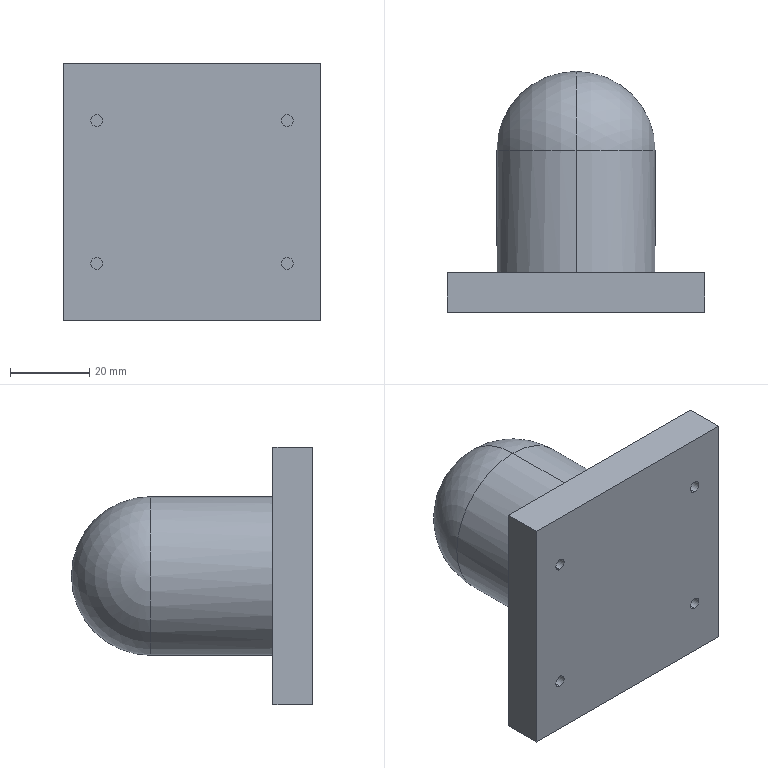Part | SolidWorks | features ICE 2, Extrusion 1, Fillet 1 | 1 solid | 22 faces | box 65 x 60.8 x 65 mm | volume 97568 mm3 | cylinder 10 | plane 10 | sphere 2 | commonest cylinder face diameters 3 x8 40 x2
STEP:
#1=CARTESIAN_POINT('',(24.,5.,-16.5));
#2=VERTEX_POINT('',#1);
#3=CARTESIAN_POINT('',(24.,5.,-19.5));
#4=VERTEX_POINT('',#3);
#5=CARTESIAN_POINT('',(24.,5.,-18.));
#6=DIRECTION('',(0.,-1.,0.));
#7=DIRECTION('',(0.,0.,-1.));
#8=AXIS2_PLACEMENT_3D('',#5,#6,#7);
#9=CIRCLE('',#8,1.5);
#10=EDGE_CURVE('',#2,#4,#9,.T.);
#11=ORIENTED_EDGE('',*,*,#10,.F.);
#12=CARTESIAN_POINT('',(24.,0.,-16.5));
#13=VERTEX_POINT('',#12);
#14=CARTESIAN_POINT('',(24.,5.,-16.5));
#15=DIRECTION('',(0.,-1.,0.));
#16=VECTOR('',#15,1000.);
#17=LINE('',#14,#16);
#18=EDGE_CURVE('',#2,#13,#17,.T.);
#19=ORIENTED_EDGE('',*,*,#18,.T.);
#20=CARTESIAN_POINT('',(24.,0.,-19.5));
#21=VERTEX_POINT('',#20);
#22=CARTESIAN_POINT('',(24.,0.,-18.));
#23=DIRECTION('',(0.,-1.,0.));
#24=DIRECTION('',(0.,0.,-1.));
#25=AXIS2_PLACEMENT_3D('',#22,#23,#24);
#26=CIRCLE('',#25,1.5);
#27=EDGE_CURVE('',#13,#21,#26,.T.);
#28=ORIENTED_EDGE('',*,*,#27,.T.);
#29=CARTESIAN_POINT('',(24.,5.,-19.5));
#30=DIRECTION('',(0.,-1.,0.));
#31=VECTOR('',#30,1000.);
#32=LINE('',#29,#31);
#33=EDGE_CURVE('',#4,#21,#32,.T.);
#34=ORIENTED_EDGE('',*,*,#33,.F.);
#35=EDGE_LOOP('',(#11,#19,#28,#34));
#36=FACE_OUTER_BOUND('',#35,.T.);
#37=CARTESIAN_POINT('',(24.,5.,-18.));
#38=DIRECTION('',(0.,-1.,0.));
#39=DIRECTION('',(0.,0.,-1.));
#40=AXIS2_PLACEMENT_3D('',#37,#38,#39);
#41=CYLINDRICAL_SURFACE('',#40,1.5);
#42=ADVANCED_FACE('',(#36),#41,.F.);
#43=CARTESIAN_POINT('',(-24.,5.,-16.5));
#44=VERTEX_POINT('',#43);
#45=CARTESIAN_POINT('',(-24.,5.,-19.5));
#46=VERTEX_POINT('',#45);
#47=CARTESIAN_POINT('',(-24.,5.,-18.));
#48=DIRECTION('',(0.,-1.,0.));
#49=DIRECTION('',(0.,0.,-1.));
#50=AXIS2_PLACEMENT_3D('',#47,#48,#49);
#51=CIRCLE('',#50,1.5);
#52=EDGE_CURVE('',#44,#46,#51,.T.);
#53=ORIENTED_EDGE('',*,*,#52,.F.);
#54=CARTESIAN_POINT('',(-24.,0.,-16.5));
#55=VERTEX_POINT('',#54);
#56=CARTESIAN_POINT('',(-24.,5.,-16.5));
#57=DIRECTION('',(0.,-1.,0.));
#58=VECTOR('',#57,1000.);
#59=LINE('',#56,#58);
#60=EDGE_CURVE('',#44,#55,#59,.T.);
#61=ORIENTED_EDGE('',*,*,#60,.T.);
#62=CARTESIAN_POINT('',(-24.,0.,-19.5));
#63=VERTEX_POINT('',#62);
#64=CARTESIAN_POINT('',(-24.,0.,-18.));
#65=DIRECTION('',(0.,-1.,0.));
#66=DIRECTION('',(0.,0.,-1.));
#67=AXIS2_PLACEMENT_3D('',#64,#65,#66);
#68=CIRCLE('',#67,1.5);
#69=EDGE_CURVE('',#55,#63,#68,.T.);
#70=ORIENTED_EDGE('',*,*,#69,.T.);
#71=CARTESIAN_POINT('',(-24.,5.,-19.5));
#72=DIRECTION('',(0.,-1.,0.));
#73=VECTOR('',#72,1000.);
#74=LINE('',#71,#73);
#75=EDGE_CURVE('',#46,#63,#74,.T.);
#76=ORIENTED_EDGE('',*,*,#75,.F.);
#77=EDGE_LOOP('',(#53,#61,#70,#76));
#78=FACE_OUTER_BOUND('',#77,.T.);
#79=CARTESIAN_POINT('',(-24.,5.,-18.));
#80=DIRECTION('',(0.,-1.,0.));
#81=DIRECTION('',(0.,0.,-1.));
#82=AXIS2_PLACEMENT_3D('',#79,#80,#81);
#83=CYLINDRICAL_SURFACE('',#82,1.5);
#84=ADVANCED_FACE('',(#78),#83,.F.);
#85=CARTESIAN_POINT('',(-24.,5.,19.5));
#86=VERTEX_POINT('',#85);
#87=CARTESIAN_POINT('',(-24.,5.,16.5));
#88=VERTEX_POINT('',#87);
#89=CARTESIAN_POINT('',(-24.,5.,18.));
#90=DIRECTION('',(0.,-1.,0.));
#91=DIRECTION('',(0.,0.,-1.));
#92=AXIS2_PLACEMENT_3D('',#89,#90,#91);
#93=CIRCLE('',#92,1.5);
#94=EDGE_CURVE('',#86,#88,#93,.T.);
#95=ORIENTED_EDGE('',*,*,#94,.F.);
#96=CARTESIAN_POINT('',(-24.,0.,19.5));
#97=VERTEX_POINT('',#96);
#98=CARTESIAN_POINT('',(-24.,5.,19.5));
#99=DIRECTION('',(0.,-1.,0.));
#100=VECTOR('',#99,1000.);
#101=LINE('',#98,#100);
#102=EDGE_CURVE('',#86,#97,#101,.T.);
#103=ORIENTED_EDGE('',*,*,#102,.T.);
#104=CARTESIAN_POINT('',(-24.,0.,16.5));
#105=VERTEX_POINT('',#104);
#106=CARTESIAN_POINT('',(-24.,0.,18.));
#107=DIRECTION('',(0.,-1.,0.));
#108=DIRECTION('',(0.,0.,-1.));
#109=AXIS2_PLACEMENT_3D('',#106,#107,#108);
#110=CIRCLE('',#109,1.5);
#111=EDGE_CURVE('',#97,#105,#110,.T.);
#112=ORIENTED_EDGE('',*,*,#111,.T.);
#113=CARTESIAN_POINT('',(-24.,5.,16.5));
#114=DIRECTION('',(0.,-1.,0.));
#115=VECTOR('',#114,1000.);
#116=LINE('',#113,#115);
#117=EDGE_CURVE('',#88,#105,#116,.T.);
#118=ORIENTED_EDGE('',*,*,#117,.F.);
#119=EDGE_LOOP('',(#95,#103,#112,#118));
#120=FACE_OUTER_BOUND('',#119,.T.);
#121=CARTESIAN_POINT('',(-24.,5.,18.));
#122=DIRECTION('',(0.,-1.,0.));
#123=DIRECTION('',(0.,0.,-1.));
#124=AXIS2_PLACEMENT_3D('',#121,#122,#123);
#125=CYLINDRICAL_SURFACE('',#124,1.5);
#126=ADVANCED_FACE('',(#120),#125,.F.);
#127=CARTESIAN_POINT('',(24.,5.,19.5));
#128=VERTEX_POINT('',#127);
#129=CARTESIAN_POINT('',(24.,5.,16.5));
#130=VERTEX_POINT('',#129);
#131=CARTESIAN_POINT('',(24.,5.,18.));
#132=DIRECTION('',(0.,-1.,0.));
#133=DIRECTION('',(0.,0.,-1.));
#134=AXIS2_PLACEMENT_3D('',#131,#132,#133);
#135=CIRCLE('',#134,1.5);
#136=EDGE_CURVE('',#128,#130,#135,.T.);
#137=ORIENTED_EDGE('',*,*,#136,.F.);
#138=CARTESIAN_POINT('',(24.,0.,19.5));
#139=VERTEX_POINT('',#138);
#140=CARTESIAN_POINT('',(24.,5.,19.5));
#141=DIRECTION('',(0.,-1.,0.));
#142=VECTOR('',#141,1000.);
#143=LINE('',#140,#142);
#144=EDGE_CURVE('',#128,#139,#143,.T.);
#145=ORIENTED_EDGE('',*,*,#144,.T.);
#146=CARTESIAN_POINT('',(24.,0.,16.5));
#147=VERTEX_POINT('',#146);
#148=CARTESIAN_POINT('',(24.,0.,18.));
#149=DIRECTION('',(0.,-1.,0.));
#150=DIRECTION('',(0.,0.,-1.));
#151=AXIS2_PLACEMENT_3D('',#148,#149,#150);
#152=CIRCLE('',#151,1.5);
#153=EDGE_CURVE('',#139,#147,#152,.T.);
#154=ORIENTED_EDGE('',*,*,#153,.T.);
#155=CARTESIAN_POINT('',(24.,5.,16.5));
#156=DIRECTION('',(0.,-1.,0.));
#157=VECTOR('',#156,1000.);
#158=LINE('',#155,#157);
#159=EDGE_CURVE('',#130,#147,#158,.T.);
#160=ORIENTED_EDGE('',*,*,#159,.F.);
#161=EDGE_LOOP('',(#137,#145,#154,#160));
#162=FACE_OUTER_BOUND('',#161,.T.);
#163=CARTESIAN_POINT('',(24.,5.,18.));
#164=DIRECTION('',(0.,-1.,0.));
#165=DIRECTION('',(0.,0.,-1.));
#166=AXIS2_PLACEMENT_3D('',#163,#164,#165);
#167=CYLINDRICAL_SURFACE('',#166,1.5);
#168=ADVANCED_FACE('',(#162),#167,.F.);
#169=CARTESIAN_POINT('',(0.,40.8,-20.));
#170=VERTEX_POINT('',#169);
#171=CARTESIAN_POINT('',(0.,40.8,20.));
#172=VERTEX_POINT('',#171);
#173=CARTESIAN_POINT('',(0.,40.8,0.));
#174=DIRECTION('',(0.,-1.,0.));
#175=DIRECTION('',(0.,0.,-1.));
#176=AXIS2_PLACEMENT_3D('',#173,#174,#175);
#177=CIRCLE('',#176,20.);
#178=EDGE_CURVE('',#170,#172,#177,.T.);
#179=ORIENTED_EDGE('',*,*,#178,.F.);
#180=CARTESIAN_POINT('',(0.,60.8,0.));
#181=VERTEX_POINT('',#180);
#182=CARTESIAN_POINT('',(0.,40.8,0.));
#183=DIRECTION('',(1.,0.,0.));
#184=DIRECTION('',(0.,0.,-1.));
#185=AXIS2_PLACEMENT_3D('',#182,#183,#184);
#186=CIRCLE('',#185,20.);
#187=EDGE_CURVE('',#170,#181,#186,.T.);
#188=ORIENTED_EDGE('',*,*,#187,.T.);
#189=CARTESIAN_POINT('',(0.,40.8,0.));
#190=DIRECTION('',(-1.,0.,0.));
#191=DIRECTION('',(0.,0.,1.));
#192=AXIS2_PLACEMENT_3D('',#189,#190,#191);
#193=CIRCLE('',#192,20.);
#194=EDGE_CURVE('',#172,#181,#193,.T.);
#195=ORIENTED_EDGE('',*,*,#194,.F.);
#196=EDGE_LOOP('',(#179,#188,#195));
#197=FACE_OUTER_BOUND('',#196,.T.);
#198=CARTESIAN_POINT('',(0.,40.8,0.));
#199=DIRECTION('',(1.,0.,0.));
#200=DIRECTION('',(0.,0.,1.));
#201=AXIS2_PLACEMENT_3D('',#198,#199,#200);
#202=SPHERICAL_SURFACE('',#201,20.);
#203=ADVANCED_FACE('',(#197),#202,.T.);
#204=ORIENTED_EDGE('',*,*,#178,.T.);
#205=CARTESIAN_POINT('',(0.,10.,20.));
#206=VERTEX_POINT('',#205);
#207=CARTESIAN_POINT('',(0.,60.8,20.));
#208=DIRECTION('',(0.,-1.,0.));
#209=VECTOR('',#208,1000.);
#210=LINE('',#207,#209);
#211=EDGE_CURVE('',#172,#206,#210,.T.);
#212=ORIENTED_EDGE('',*,*,#211,.T.);
#213=CARTESIAN_POINT('',(0.,10.,-20.));
#214=VERTEX_POINT('',#213);
#215=CARTESIAN_POINT('',(0.,10.,0.));
#216=DIRECTION('',(0.,1.,0.));
#217=DIRECTION('',(0.,0.,1.));
#218=AXIS2_PLACEMENT_3D('',#215,#216,#217);
#219=CIRCLE('',#218,20.);
#220=EDGE_CURVE('',#206,#214,#219,.T.);
#221=ORIENTED_EDGE('',*,*,#220,.T.);
#222=CARTESIAN_POINT('',(0.,60.8,-20.));
#223=DIRECTION('',(0.,-1.,0.));
#224=VECTOR('',#223,1000.);
#225=LINE('',#222,#224);
#226=EDGE_CURVE('',#170,#214,#225,.T.);
#227=ORIENTED_EDGE('',*,*,#226,.F.);
#228=EDGE_LOOP('',(#204,#212,#221,#227));
#229=FACE_OUTER_BOUND('',#228,.T.);
#230=CARTESIAN_POINT('',(0.,60.8,0.));
#231=DIRECTION('',(0.,-1.,0.));
#232=DIRECTION('',(0.,0.,-1.));
#233=AXIS2_PLACEMENT_3D('',#230,#231,#232);
#234=CYLINDRICAL_SURFACE('',#233,20.);
#235=ADVANCED_FACE('',(#229),#234,.T.);
#236=CARTESIAN_POINT('',(32.5,0.,32.5));
#237=VERTEX_POINT('',#236);
#238=CARTESIAN_POINT('',(32.5,0.,-32.5));
#239=VERTEX_POINT('',#238);
#240=CARTESIAN_POINT('',(32.5,0.,32.5));
#241=DIRECTION('',(0.,0.,-1.));
#242=VECTOR('',#241,1000.);
#243=LINE('',#240,#242);
#244=EDGE_CURVE('',#237,#239,#243,.T.);
#245=ORIENTED_EDGE('',*,*,#244,.T.);
#246=CARTESIAN_POINT('',(32.5,10.,-32.5));
#247=VERTEX_POINT('',#246);
#248=CARTESIAN_POINT('',(32.5,10.,-32.5));
#249=DIRECTION('',(0.,-1.,0.));
#250=VECTOR('',#249,1000.);
#251=LINE('',#248,#250);
#252=EDGE_CURVE('',#247,#239,#251,.T.);
#253=ORIENTED_EDGE('',*,*,#252,.F.);
#254=CARTESIAN_POINT('',(32.5,10.,32.5));
#255=VERTEX_POINT('',#254);
#256=CARTESIAN_POINT('',(32.5,10.,32.5));
#257=DIRECTION('',(0.,0.,-1.));
#258=VECTOR('',#257,1000.);
#259=LINE('',#256,#258);
#260=EDGE_CURVE('',#255,#247,#259,.T.);
#261=ORIENTED_EDGE('',*,*,#260,.F.);
#262=CARTESIAN_POINT('',(32.5,10.,32.5));
#263=DIRECTION('',(0.,-1.,0.));
#264=VECTOR('',#263,1000.);
#265=LINE('',#262,#264);
#266=EDGE_CURVE('',#255,#237,#265,.T.);
#267=ORIENTED_EDGE('',*,*,#266,.T.);
#268=EDGE_LOOP('',(#245,#253,#261,#267));
#269=FACE_OUTER_BOUND('',#268,.T.);
#270=CARTESIAN_POINT('',(32.5,10.,32.5));
#271=DIRECTION('',(-1.,0.,0.));
#272=DIRECTION('',(0.,0.,1.));
#273=AXIS2_PLACEMENT_3D('',#270,#271,#272);
#274=PLANE('',#273);
#275=ADVANCED_FACE('',(#269),#274,.F.);
#276=CARTESIAN_POINT('',(-32.5,0.,-32.5));
#277=VERTEX_POINT('',#276);
#278=CARTESIAN_POINT('',(-32.5,0.,-32.5));
#279=DIRECTION('',(-1.,0.,0.));
#280=VECTOR('',#279,1000.);
#281=LINE('',#278,#280);
#282=EDGE_CURVE('',#239,#277,#281,.T.);
#283=ORIENTED_EDGE('',*,*,#282,.T.);
#284=CARTESIAN_POINT('',(-32.5,10.,-32.5));
#285=VERTEX_POINT('',#284);
#286=CARTESIAN_POINT('',(-32.5,10.,-32.5));
#287=DIRECTION('',(0.,-1.,0.));
#288=VECTOR('',#287,1000.);
#289=LINE('',#286,#288);
#290=EDGE_CURVE('',#285,#277,#289,.T.);
#291=ORIENTED_EDGE('',*,*,#290,.F.);
#292=CARTESIAN_POINT('',(-32.5,10.,-32.5));
#293=DIRECTION('',(-1.,0.,0.));
#294=VECTOR('',#293,1000.);
#295=LINE('',#292,#294);
#296=EDGE_CURVE('',#247,#285,#295,.T.);
#297=ORIENTED_EDGE('',*,*,#296,.F.);
#298=ORIENTED_EDGE('',*,*,#252,.T.);
#299=EDGE_LOOP('',(#283,#291,#297,#298));
#300=FACE_OUTER_BOUND('',#299,.T.);
#301=CARTESIAN_POINT('',(-32.5,10.,-32.5));
#302=DIRECTION('',(0.,0.,1.));
#303=DIRECTION('',(1.,0.,0.));
#304=AXIS2_PLACEMENT_3D('',#301,#302,#303);
#305=PLANE('',#304);
#306=ADVANCED_FACE('',(#300),#305,.F.);
#307=CARTESIAN_POINT('',(-32.5,0.,32.5));
#308=VERTEX_POINT('',#307);
#309=CARTESIAN_POINT('',(-32.5,0.,32.5));
#310=DIRECTION('',(0.,0.,1.));
#311=VECTOR('',#310,1000.);
#312=LINE('',#309,#311);
#313=EDGE_CURVE('',#277,#308,#312,.T.);
#314=ORIENTED_EDGE('',*,*,#313,.T.);
#315=CARTESIAN_POINT('',(-32.5,10.,32.5));
#316=VERTEX_POINT('',#315);
#317=CARTESIAN_POINT('',(-32.5,10.,32.5));
#318=DIRECTION('',(0.,-1.,0.));
#319=VECTOR('',#318,1000.);
#320=LINE('',#317,#319);
#321=EDGE_CURVE('',#316,#308,#320,.T.);
#322=ORIENTED_EDGE('',*,*,#321,.F.);
#323=CARTESIAN_POINT('',(-32.5,10.,32.5));
#324=DIRECTION('',(0.,0.,1.));
#325=VECTOR('',#324,1000.);
#326=LINE('',#323,#325);
#327=EDGE_CURVE('',#285,#316,#326,.T.);
#328=ORIENTED_EDGE('',*,*,#327,.F.);
#329=ORIENTED_EDGE('',*,*,#290,.T.);
#330=EDGE_LOOP('',(#314,#322,#328,#329));
#331=FACE_OUTER_BOUND('',#330,.T.);
#332=CARTESIAN_POINT('',(-32.5,10.,32.5));
#333=DIRECTION('',(1.,0.,0.));
#334=DIRECTION('',(0.,0.,-1.));
#335=AXIS2_PLACEMENT_3D('',#332,#333,#334);
#336=PLANE('',#335);
#337=ADVANCED_FACE('',(#331),#336,.F.);
#338=CARTESIAN_POINT('',(-32.5,0.,32.5));
#339=DIRECTION('',(1.,0.,0.));
#340=VECTOR('',#339,1000.);
#341=LINE('',#338,#340);
#342=EDGE_CURVE('',#308,#237,#341,.T.);
#343=ORIENTED_EDGE('',*,*,#342,.T.);
#344=ORIENTED_EDGE('',*,*,#266,.F.);
#345=CARTESIAN_POINT('',(-32.5,10.,32.5));
#346=DIRECTION('',(1.,0.,0.));
#347=VECTOR('',#346,1000.);
#348=LINE('',#345,#347);
#349=EDGE_CURVE('',#316,#255,#348,.T.);
#350=ORIENTED_EDGE('',*,*,#349,.F.);
#351=ORIENTED_EDGE('',*,*,#321,.T.);
#352=EDGE_LOOP('',(#343,#344,#350,#351));
#353=FACE_OUTER_BOUND('',#352,.T.);
#354=CARTESIAN_POINT('',(-32.5,10.,32.5));
#355=DIRECTION('',(0.,0.,-1.));
#356=DIRECTION('',(-1.,0.,0.));
#357=AXIS2_PLACEMENT_3D('',#354,#355,#356);
#358=PLANE('',#357);
#359=ADVANCED_FACE('',(#353),#358,.F.);
#360=CARTESIAN_POINT('',(0.,10.,0.));
#361=DIRECTION('',(0.,1.,0.));
#362=DIRECTION('',(0.,0.,1.));
#363=AXIS2_PLACEMENT_3D('',#360,#361,#362);
#364=CIRCLE('',#363,20.);
#365=EDGE_CURVE('',#214,#206,#364,.T.);
#366=ORIENTED_EDGE('',*,*,#365,.F.);
#367=ORIENTED_EDGE('',*,*,#220,.F.);
#368=EDGE_LOOP('',(#366,#367));
#369=FACE_BOUND('',#368,.T.);
#370=ORIENTED_EDGE('',*,*,#260,.T.);
#371=ORIENTED_EDGE('',*,*,#296,.T.);
#372=ORIENTED_EDGE('',*,*,#327,.T.);
#373=ORIENTED_EDGE('',*,*,#349,.T.);
#374=EDGE_LOOP('',(#370,#371,#372,#373));
#375=FACE_OUTER_BOUND('',#374,.T.);
#376=CARTESIAN_POINT('',(0.,10.,0.));
#377=DIRECTION('',(0.,-1.,0.));
#378=DIRECTION('',(0.,0.,-1.));
#379=AXIS2_PLACEMENT_3D('',#376,#377,#378);
#380=PLANE('',#379);
#381=ADVANCED_FACE('',(#369,#375),#380,.F.);
#382=CARTESIAN_POINT('',(24.,0.,-18.));
#383=DIRECTION('',(0.,-1.,0.));
#384=DIRECTION('',(0.,0.,-1.));
#385=AXIS2_PLACEMENT_3D('',#382,#383,#384);
#386=CIRCLE('',#385,1.5);
#387=EDGE_CURVE('',#21,#13,#386,.T.);
#388=ORIENTED_EDGE('',*,*,#387,.F.);
#389=ORIENTED_EDGE('',*,*,#27,.F.);
#390=EDGE_LOOP('',(#388,#389));
#391=FACE_BOUND('',#390,.T.);
#392=CARTESIAN_POINT('',(-24.,0.,-18.));
#393=DIRECTION('',(0.,-1.,0.));
#394=DIRECTION('',(0.,0.,-1.));
#395=AXIS2_PLACEMENT_3D('',#392,#393,#394);
#396=CIRCLE('',#395,1.5);
#397=EDGE_CURVE('',#63,#55,#396,.T.);
#398=ORIENTED_EDGE('',*,*,#397,.F.);
#399=ORIENTED_EDGE('',*,*,#69,.F.);
#400=EDGE_LOOP('',(#398,#399));
#401=FACE_BOUND('',#400,.T.);
#402=CARTESIAN_POINT('',(-24.,0.,18.));
#403=DIRECTION('',(0.,-1.,0.));
#404=DIRECTION('',(0.,0.,-1.));
#405=AXIS2_PLACEMENT_3D('',#402,#403,#404);
#406=CIRCLE('',#405,1.5);
#407=EDGE_CURVE('',#105,#97,#406,.T.);
#408=ORIENTED_EDGE('',*,*,#407,.F.);
#409=ORIENTED_EDGE('',*,*,#111,.F.);
#410=EDGE_LOOP('',(#408,#409));
#411=FACE_BOUND('',#410,.T.);
#412=CARTESIAN_POINT('',(24.,0.,18.));
#413=DIRECTION('',(0.,-1.,0.));
#414=DIRECTION('',(0.,0.,-1.));
#415=AXIS2_PLACEMENT_3D('',#412,#413,#414);
#416=CIRCLE('',#415,1.5);
#417=EDGE_CURVE('',#147,#139,#416,.T.);
#418=ORIENTED_EDGE('',*,*,#417,.F.);
#419=ORIENTED_EDGE('',*,*,#153,.F.);
#420=EDGE_LOOP('',(#418,#419));
#421=FACE_BOUND('',#420,.T.);
#422=ORIENTED_EDGE('',*,*,#244,.F.);
#423=ORIENTED_EDGE('',*,*,#342,.F.);
#424=ORIENTED_EDGE('',*,*,#313,.F.);
#425=ORIENTED_EDGE('',*,*,#282,.F.);
#426=EDGE_LOOP('',(#422,#423,#424,#425));
#427=FACE_OUTER_BOUND('',#426,.T.);
#428=CARTESIAN_POINT('',(0.,0.,0.));
#429=DIRECTION('',(0.,-1.,0.));
#430=DIRECTION('',(0.,0.,-1.));
#431=AXIS2_PLACEMENT_3D('',#428,#429,#430);
#432=PLANE('',#431);
#433=ADVANCED_FACE('',(#391,#401,#411,#421,#427),#432,.T.);
#434=ORIENTED_EDGE('',*,*,#211,.F.);
#435=CARTESIAN_POINT('',(0.,40.8,0.));
#436=DIRECTION('',(0.,-1.,0.));
#437=DIRECTION('',(0.,0.,-1.));
#438=AXIS2_PLACEMENT_3D('',#435,#436,#437);
#439=CIRCLE('',#438,20.);
#440=EDGE_CURVE('',#172,#170,#439,.T.);
#441=ORIENTED_EDGE('',*,*,#440,.T.);
#442=ORIENTED_EDGE('',*,*,#226,.T.);
#443=ORIENTED_EDGE('',*,*,#365,.T.);
#444=EDGE_LOOP('',(#434,#441,#442,#443));
#445=FACE_OUTER_BOUND('',#444,.T.);
#446=CARTESIAN_POINT('',(0.,60.8,0.));
#447=DIRECTION('',(0.,-1.,0.));
#448=DIRECTION('',(0.,0.,-1.));
#449=AXIS2_PLACEMENT_3D('',#446,#447,#448);
#450=CYLINDRICAL_SURFACE('',#449,20.);
#451=ADVANCED_FACE('',(#445),#450,.T.);
#452=ORIENTED_EDGE('',*,*,#187,.F.);
#453=ORIENTED_EDGE('',*,*,#440,.F.);
#454=ORIENTED_EDGE('',*,*,#194,.T.);
#455=EDGE_LOOP('',(#452,#453,#454));
#456=FACE_OUTER_BOUND('',#455,.T.);
#457=CARTESIAN_POINT('',(0.,40.8,0.));
#458=DIRECTION('',(1.,0.,0.));
#459=DIRECTION('',(0.,0.,1.));
#460=AXIS2_PLACEMENT_3D('',#457,#458,#459);
#461=SPHERICAL_SURFACE('',#460,20.);
#462=ADVANCED_FACE('',(#456),#461,.T.);
#463=ORIENTED_EDGE('',*,*,#144,.F.);
#464=CARTESIAN_POINT('',(24.,5.,18.));
#465=DIRECTION('',(0.,-1.,0.));
#466=DIRECTION('',(0.,0.,-1.));
#467=AXIS2_PLACEMENT_3D('',#464,#465,#466);
#468=CIRCLE('',#467,1.5);
#469=EDGE_CURVE('',#130,#128,#468,.T.);
#470=ORIENTED_EDGE('',*,*,#469,.F.);
#471=ORIENTED_EDGE('',*,*,#159,.T.);
#472=ORIENTED_EDGE('',*,*,#417,.T.);
#473=EDGE_LOOP('',(#463,#470,#471,#472));
#474=FACE_OUTER_BOUND('',#473,.T.);
#475=CARTESIAN_POINT('',(24.,5.,18.));
#476=DIRECTION('',(0.,-1.,0.));
#477=DIRECTION('',(0.,0.,-1.));
#478=AXIS2_PLACEMENT_3D('',#475,#476,#477);
#479=CYLINDRICAL_SURFACE('',#478,1.5);
#480=ADVANCED_FACE('',(#474),#479,.F.);
#481=ORIENTED_EDGE('',*,*,#469,.T.);
#482=ORIENTED_EDGE('',*,*,#136,.T.);
#483=EDGE_LOOP('',(#481,#482));
#484=FACE_OUTER_BOUND('',#483,.T.);
#485=CARTESIAN_POINT('',(24.,5.,18.));
#486=DIRECTION('',(0.,-1.,0.));
#487=DIRECTION('',(0.,0.,-1.));
#488=AXIS2_PLACEMENT_3D('',#485,#486,#487);
#489=PLANE('',#488);
#490=ADVANCED_FACE('',(#484),#489,.T.);
#491=ORIENTED_EDGE('',*,*,#102,.F.);
#492=CARTESIAN_POINT('',(-24.,5.,18.));
#493=DIRECTION('',(0.,-1.,0.));
#494=DIRECTION('',(0.,0.,-1.));
#495=AXIS2_PLACEMENT_3D('',#492,#493,#494);
#496=CIRCLE('',#495,1.5);
#497=EDGE_CURVE('',#88,#86,#496,.T.);
#498=ORIENTED_EDGE('',*,*,#497,.F.);
#499=ORIENTED_EDGE('',*,*,#117,.T.);
#500=ORIENTED_EDGE('',*,*,#407,.T.);
#501=EDGE_LOOP('',(#491,#498,#499,#500));
#502=FACE_OUTER_BOUND('',#501,.T.);
#503=CARTESIAN_POINT('',(-24.,5.,18.));
#504=DIRECTION('',(0.,-1.,0.));
#505=DIRECTION('',(0.,0.,-1.));
#506=AXIS2_PLACEMENT_3D('',#503,#504,#505);
#507=CYLINDRICAL_SURFACE('',#506,1.5);
#508=ADVANCED_FACE('',(#502),#507,.F.);
#509=ORIENTED_EDGE('',*,*,#497,.T.);
#510=ORIENTED_EDGE('',*,*,#94,.T.);
#511=EDGE_LOOP('',(#509,#510));
#512=FACE_OUTER_BOUND('',#511,.T.);
#513=CARTESIAN_POINT('',(-24.,5.,18.));
#514=DIRECTION('',(0.,-1.,0.));
#515=DIRECTION('',(0.,0.,-1.));
#516=AXIS2_PLACEMENT_3D('',#513,#514,#515);
#517=PLANE('',#516);
#518=ADVANCED_FACE('',(#512),#517,.T.);
#519=ORIENTED_EDGE('',*,*,#60,.F.);
#520=CARTESIAN_POINT('',(-24.,5.,-18.));
#521=DIRECTION('',(0.,-1.,0.));
#522=DIRECTION('',(0.,0.,-1.));
#523=AXIS2_PLACEMENT_3D('',#520,#521,#522);
#524=CIRCLE('',#523,1.5);
#525=EDGE_CURVE('',#46,#44,#524,.T.);
#526=ORIENTED_EDGE('',*,*,#525,.F.);
#527=ORIENTED_EDGE('',*,*,#75,.T.);
#528=ORIENTED_EDGE('',*,*,#397,.T.);
#529=EDGE_LOOP('',(#519,#526,#527,#528));
#530=FACE_OUTER_BOUND('',#529,.T.);
#531=CARTESIAN_POINT('',(-24.,5.,-18.));
#532=DIRECTION('',(0.,-1.,0.));
#533=DIRECTION('',(0.,0.,-1.));
#534=AXIS2_PLACEMENT_3D('',#531,#532,#533);
#535=CYLINDRICAL_SURFACE('',#534,1.5);
#536=ADVANCED_FACE('',(#530),#535,.F.);
#537=ORIENTED_EDGE('',*,*,#525,.T.);
#538=ORIENTED_EDGE('',*,*,#52,.T.);
#539=EDGE_LOOP('',(#537,#538));
#540=FACE_OUTER_BOUND('',#539,.T.);
#541=CARTESIAN_POINT('',(-24.,5.,-18.));
#542=DIRECTION('',(0.,-1.,0.));
#543=DIRECTION('',(0.,0.,-1.));
#544=AXIS2_PLACEMENT_3D('',#541,#542,#543);
#545=PLANE('',#544);
#546=ADVANCED_FACE('',(#540),#545,.T.);
#547=ORIENTED_EDGE('',*,*,#18,.F.);
#548=CARTESIAN_POINT('',(24.,5.,-18.));
#549=DIRECTION('',(0.,-1.,0.));
#550=DIRECTION('',(0.,0.,-1.));
#551=AXIS2_PLACEMENT_3D('',#548,#549,#550);
#552=CIRCLE('',#551,1.5);
#553=EDGE_CURVE('',#4,#2,#552,.T.);
#554=ORIENTED_EDGE('',*,*,#553,.F.);
#555=ORIENTED_EDGE('',*,*,#33,.T.);
#556=ORIENTED_EDGE('',*,*,#387,.T.);
#557=EDGE_LOOP('',(#547,#554,#555,#556));
#558=FACE_OUTER_BOUND('',#557,.T.);
#559=CARTESIAN_POINT('',(24.,5.,-18.));
#560=DIRECTION('',(0.,-1.,0.));
#561=DIRECTION('',(0.,0.,-1.));
#562=AXIS2_PLACEMENT_3D('',#559,#560,#561);
#563=CYLINDRICAL_SURFACE('',#562,1.5);
#564=ADVANCED_FACE('',(#558),#563,.F.);
#565=ORIENTED_EDGE('',*,*,#553,.T.);
#566=ORIENTED_EDGE('',*,*,#10,.T.);
#567=EDGE_LOOP('',(#565,#566));
#568=FACE_OUTER_BOUND('',#567,.T.);
#569=CARTESIAN_POINT('',(24.,5.,-18.));
#570=DIRECTION('',(0.,-1.,0.));
#571=DIRECTION('',(0.,0.,-1.));
#572=AXIS2_PLACEMENT_3D('',#569,#570,#571);
#573=PLANE('',#572);
#574=ADVANCED_FACE('',(#568),#573,.T.);
#575=CLOSED_SHELL('',(#42,#84,#126,#168,#203,#235,#275,#306,#337,#359,#381,#433,#451,#462,#480,#490,#508,#518,#536,#546,#564,#574));
#576=MANIFOLD_SOLID_BREP('',#575);
#577=CARTESIAN_POINT('',(0.,0.,0.));
#578=DIRECTION('',(0.,0.,1.));
#579=DIRECTION('',(1.,0.,0.));
#580=AXIS2_PLACEMENT_3D('',#577,#578,#579);
#581=(LENGTH_UNIT()NAMED_UNIT(*)SI_UNIT(.MILLI.,.METRE.));
#582=UNCERTAINTY_MEASURE_WITH_UNIT(LENGTH_MEASURE(0.00001),#581,'','');
#583=(NAMED_UNIT(*)PLANE_ANGLE_UNIT()SI_UNIT($,.RADIAN.));
#584=(NAMED_UNIT(*)SI_UNIT($,.STERADIAN.)SOLID_ANGLE_UNIT());
#585=(GEOMETRIC_REPRESENTATION_CONTEXT(3)GLOBAL_UNCERTAINTY_ASSIGNED_CONTEXT((#582))GLOBAL_UNIT_ASSIGNED_CONTEXT((#581,#583,#584))REPRESENTATION_CONTEXT('',''));
#586=ADVANCED_BREP_SHAPE_REPRESENTATION('',(#576,#580),#585);